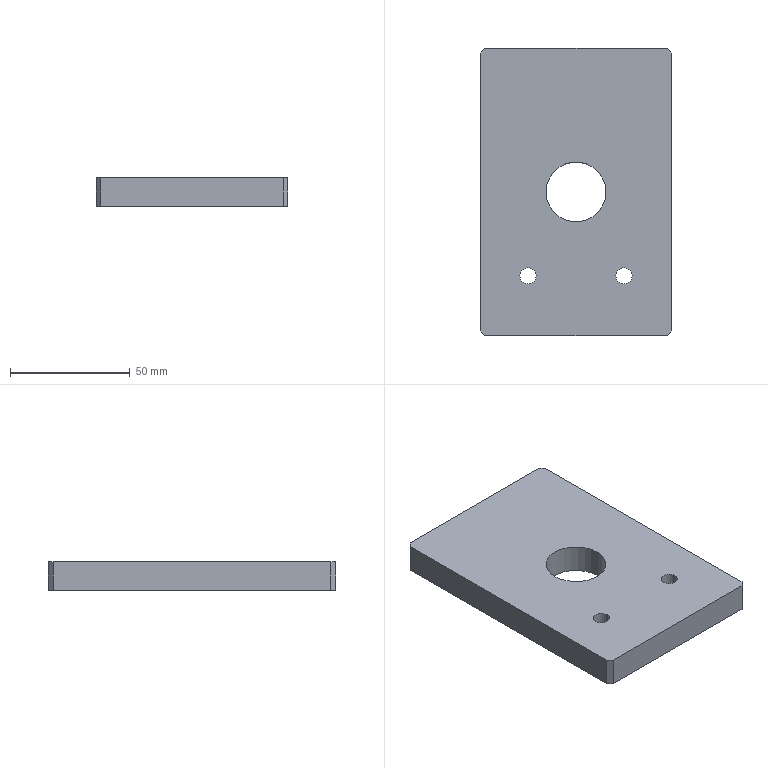Part | SolidWorks | features BaseBody 1 | 1 solid | 24 faces | box 80 x 120 x 12 mm | volume 106676 mm3 | cylinder 10 | plane 10 | cone 4 | commonest cylinder face diameters 6.8 x8 25 x2
STEP:
#1=CARTESIAN_POINT('',(12.5,0.,0.));
#2=VERTEX_POINT('',#1);
#3=CARTESIAN_POINT('',(-12.5,0.,0.));
#4=VERTEX_POINT('',#3);
#5=CARTESIAN_POINT('',(0.,0.,0.));
#6=DIRECTION('',(0.,0.,-1.));
#7=DIRECTION('',(1.,0.,0.));
#8=AXIS2_PLACEMENT_3D('',#5,#6,#7);
#9=CIRCLE('',#8,12.5);
#10=EDGE_CURVE('',#2,#4,#9,.T.);
#11=ORIENTED_EDGE('',*,*,#10,.T.);
#12=CARTESIAN_POINT('',(-12.5,0.,12.));
#13=VERTEX_POINT('',#12);
#14=CARTESIAN_POINT('',(-12.5,0.,0.));
#15=DIRECTION('',(0.,0.,1.));
#16=VECTOR('',#15,1000.);
#17=LINE('',#14,#16);
#18=EDGE_CURVE('',#4,#13,#17,.T.);
#19=ORIENTED_EDGE('',*,*,#18,.T.);
#20=CARTESIAN_POINT('',(12.5,0.,12.));
#21=VERTEX_POINT('',#20);
#22=CARTESIAN_POINT('',(0.,0.,12.));
#23=DIRECTION('',(0.,0.,-1.));
#24=DIRECTION('',(1.,0.,0.));
#25=AXIS2_PLACEMENT_3D('',#22,#23,#24);
#26=CIRCLE('',#25,12.5);
#27=EDGE_CURVE('',#21,#13,#26,.T.);
#28=ORIENTED_EDGE('',*,*,#27,.F.);
#29=CARTESIAN_POINT('',(12.5,0.,0.));
#30=DIRECTION('',(0.,0.,1.));
#31=VECTOR('',#30,1000.);
#32=LINE('',#29,#31);
#33=EDGE_CURVE('',#2,#21,#32,.T.);
#34=ORIENTED_EDGE('',*,*,#33,.F.);
#35=EDGE_LOOP('',(#11,#19,#28,#34));
#36=FACE_OUTER_BOUND('',#35,.T.);
#37=CARTESIAN_POINT('',(0.,0.,0.));
#38=DIRECTION('',(0.,0.,1.));
#39=DIRECTION('',(1.,0.,0.));
#40=AXIS2_PLACEMENT_3D('',#37,#38,#39);
#41=CYLINDRICAL_SURFACE('',#40,12.5);
#42=ADVANCED_FACE('',(#36),#41,.F.);
#43=CARTESIAN_POINT('',(-16.6,-35.,12.));
#44=VERTEX_POINT('',#43);
#45=CARTESIAN_POINT('',(-23.4,-35.,12.));
#46=VERTEX_POINT('',#45);
#47=CARTESIAN_POINT('',(-20.,-35.,12.));
#48=DIRECTION('',(0.,0.,-1.));
#49=DIRECTION('',(-1.,0.,0.));
#50=AXIS2_PLACEMENT_3D('',#47,#48,#49);
#51=CIRCLE('',#50,3.4);
#52=EDGE_CURVE('',#44,#46,#51,.T.);
#53=ORIENTED_EDGE('',*,*,#52,.F.);
#54=CARTESIAN_POINT('',(-16.6,-35.,0.));
#55=VERTEX_POINT('',#54);
#56=CARTESIAN_POINT('',(-16.6,-35.,0.));
#57=DIRECTION('',(0.,0.,-1.));
#58=VECTOR('',#57,1000.);
#59=LINE('',#56,#58);
#60=EDGE_CURVE('',#44,#55,#59,.T.);
#61=ORIENTED_EDGE('',*,*,#60,.T.);
#62=CARTESIAN_POINT('',(-23.4,-35.,0.));
#63=VERTEX_POINT('',#62);
#64=CARTESIAN_POINT('',(-20.,-35.,0.));
#65=DIRECTION('',(0.,0.,-1.));
#66=DIRECTION('',(-1.,0.,0.));
#67=AXIS2_PLACEMENT_3D('',#64,#65,#66);
#68=CIRCLE('',#67,3.4);
#69=EDGE_CURVE('',#55,#63,#68,.T.);
#70=ORIENTED_EDGE('',*,*,#69,.T.);
#71=CARTESIAN_POINT('',(-23.4,-35.,0.));
#72=DIRECTION('',(0.,0.,-1.));
#73=VECTOR('',#72,1000.);
#74=LINE('',#71,#73);
#75=EDGE_CURVE('',#46,#63,#74,.T.);
#76=ORIENTED_EDGE('',*,*,#75,.F.);
#77=EDGE_LOOP('',(#53,#61,#70,#76));
#78=FACE_OUTER_BOUND('',#77,.T.);
#79=CARTESIAN_POINT('',(-20.,-35.,0.));
#80=DIRECTION('',(0.,0.,-1.));
#81=DIRECTION('',(-1.,0.,0.));
#82=AXIS2_PLACEMENT_3D('',#79,#80,#81);
#83=CYLINDRICAL_SURFACE('',#82,3.4);
#84=ADVANCED_FACE('',(#78),#83,.F.);
#85=CARTESIAN_POINT('',(23.4,-35.,12.));
#86=VERTEX_POINT('',#85);
#87=CARTESIAN_POINT('',(16.6,-35.,12.));
#88=VERTEX_POINT('',#87);
#89=CARTESIAN_POINT('',(20.,-35.,12.));
#90=DIRECTION('',(0.,0.,-1.));
#91=DIRECTION('',(-1.,0.,0.));
#92=AXIS2_PLACEMENT_3D('',#89,#90,#91);
#93=CIRCLE('',#92,3.4);
#94=EDGE_CURVE('',#86,#88,#93,.T.);
#95=ORIENTED_EDGE('',*,*,#94,.F.);
#96=CARTESIAN_POINT('',(23.4,-35.,0.));
#97=VERTEX_POINT('',#96);
#98=CARTESIAN_POINT('',(23.4,-35.,0.));
#99=DIRECTION('',(0.,0.,-1.));
#100=VECTOR('',#99,1000.);
#101=LINE('',#98,#100);
#102=EDGE_CURVE('',#86,#97,#101,.T.);
#103=ORIENTED_EDGE('',*,*,#102,.T.);
#104=CARTESIAN_POINT('',(16.6,-35.,0.));
#105=VERTEX_POINT('',#104);
#106=CARTESIAN_POINT('',(20.,-35.,0.));
#107=DIRECTION('',(0.,0.,-1.));
#108=DIRECTION('',(-1.,0.,0.));
#109=AXIS2_PLACEMENT_3D('',#106,#107,#108);
#110=CIRCLE('',#109,3.4);
#111=EDGE_CURVE('',#97,#105,#110,.T.);
#112=ORIENTED_EDGE('',*,*,#111,.T.);
#113=CARTESIAN_POINT('',(16.6,-35.,0.));
#114=DIRECTION('',(0.,0.,-1.));
#115=VECTOR('',#114,1000.);
#116=LINE('',#113,#115);
#117=EDGE_CURVE('',#88,#105,#116,.T.);
#118=ORIENTED_EDGE('',*,*,#117,.F.);
#119=EDGE_LOOP('',(#95,#103,#112,#118));
#120=FACE_OUTER_BOUND('',#119,.T.);
#121=CARTESIAN_POINT('',(20.,-35.,0.));
#122=DIRECTION('',(0.,0.,-1.));
#123=DIRECTION('',(-1.,0.,0.));
#124=AXIS2_PLACEMENT_3D('',#121,#122,#123);
#125=CYLINDRICAL_SURFACE('',#124,3.4);
#126=ADVANCED_FACE('',(#120),#125,.F.);
#127=CARTESIAN_POINT('',(-20.,37.75,2.6));
#128=VERTEX_POINT('',#127);
#129=CARTESIAN_POINT('',(-20.,37.75,9.4));
#130=VERTEX_POINT('',#129);
#131=CARTESIAN_POINT('',(-20.,37.75,6.));
#132=DIRECTION('',(0.,1.,0.));
#133=DIRECTION('',(0.,0.,1.));
#134=AXIS2_PLACEMENT_3D('',#131,#132,#133);
#135=CIRCLE('',#134,3.4);
#136=EDGE_CURVE('',#128,#130,#135,.T.);
#137=ORIENTED_EDGE('',*,*,#136,.F.);
#138=CARTESIAN_POINT('',(-20.,60.,2.6));
#139=VERTEX_POINT('',#138);
#140=CARTESIAN_POINT('',(-20.,60.,2.6));
#141=DIRECTION('',(0.,1.,0.));
#142=VECTOR('',#141,1000.);
#143=LINE('',#140,#142);
#144=EDGE_CURVE('',#128,#139,#143,.T.);
#145=ORIENTED_EDGE('',*,*,#144,.T.);
#146=CARTESIAN_POINT('',(-20.,60.,9.4));
#147=VERTEX_POINT('',#146);
#148=CARTESIAN_POINT('',(-20.,60.,6.));
#149=DIRECTION('',(0.,1.,0.));
#150=DIRECTION('',(0.,0.,1.));
#151=AXIS2_PLACEMENT_3D('',#148,#149,#150);
#152=CIRCLE('',#151,3.4);
#153=EDGE_CURVE('',#139,#147,#152,.T.);
#154=ORIENTED_EDGE('',*,*,#153,.T.);
#155=CARTESIAN_POINT('',(-20.,60.,9.4));
#156=DIRECTION('',(0.,1.,0.));
#157=VECTOR('',#156,1000.);
#158=LINE('',#155,#157);
#159=EDGE_CURVE('',#130,#147,#158,.T.);
#160=ORIENTED_EDGE('',*,*,#159,.F.);
#161=EDGE_LOOP('',(#137,#145,#154,#160));
#162=FACE_OUTER_BOUND('',#161,.T.);
#163=CARTESIAN_POINT('',(-20.,60.,6.));
#164=DIRECTION('',(0.,1.,0.));
#165=DIRECTION('',(0.,0.,1.));
#166=AXIS2_PLACEMENT_3D('',#163,#164,#165);
#167=CYLINDRICAL_SURFACE('',#166,3.4);
#168=ADVANCED_FACE('',(#162),#167,.F.);
#169=CARTESIAN_POINT('',(20.,37.75,2.6));
#170=VERTEX_POINT('',#169);
#171=CARTESIAN_POINT('',(20.,37.75,9.4));
#172=VERTEX_POINT('',#171);
#173=CARTESIAN_POINT('',(20.,37.75,6.));
#174=DIRECTION('',(0.,1.,0.));
#175=DIRECTION('',(0.,0.,1.));
#176=AXIS2_PLACEMENT_3D('',#173,#174,#175);
#177=CIRCLE('',#176,3.4);
#178=EDGE_CURVE('',#170,#172,#177,.T.);
#179=ORIENTED_EDGE('',*,*,#178,.F.);
#180=CARTESIAN_POINT('',(20.,60.,2.6));
#181=VERTEX_POINT('',#180);
#182=CARTESIAN_POINT('',(20.,60.,2.6));
#183=DIRECTION('',(0.,1.,0.));
#184=VECTOR('',#183,1000.);
#185=LINE('',#182,#184);
#186=EDGE_CURVE('',#170,#181,#185,.T.);
#187=ORIENTED_EDGE('',*,*,#186,.T.);
#188=CARTESIAN_POINT('',(20.,60.,9.4));
#189=VERTEX_POINT('',#188);
#190=CARTESIAN_POINT('',(20.,60.,6.));
#191=DIRECTION('',(0.,1.,0.));
#192=DIRECTION('',(0.,0.,1.));
#193=AXIS2_PLACEMENT_3D('',#190,#191,#192);
#194=CIRCLE('',#193,3.4);
#195=EDGE_CURVE('',#181,#189,#194,.T.);
#196=ORIENTED_EDGE('',*,*,#195,.T.);
#197=CARTESIAN_POINT('',(20.,60.,9.4));
#198=DIRECTION('',(0.,1.,0.));
#199=VECTOR('',#198,1000.);
#200=LINE('',#197,#199);
#201=EDGE_CURVE('',#172,#189,#200,.T.);
#202=ORIENTED_EDGE('',*,*,#201,.F.);
#203=EDGE_LOOP('',(#179,#187,#196,#202));
#204=FACE_OUTER_BOUND('',#203,.T.);
#205=CARTESIAN_POINT('',(20.,60.,6.));
#206=DIRECTION('',(0.,1.,0.));
#207=DIRECTION('',(0.,0.,1.));
#208=AXIS2_PLACEMENT_3D('',#205,#206,#207);
#209=CYLINDRICAL_SURFACE('',#208,3.4);
#210=ADVANCED_FACE('',(#204),#209,.F.);
#211=CARTESIAN_POINT('',(-20.,35.707,6.));
#212=VERTEX_POINT('',#211);
#213=CARTESIAN_POINT('',(-20.,37.75,9.4));
#214=DIRECTION('',(0.,0.515,0.8572));
#215=VECTOR('',#214,1000.);
#216=LINE('',#213,#215);
#217=EDGE_CURVE('',#212,#130,#216,.T.);
#218=ORIENTED_EDGE('',*,*,#217,.F.);
#219=CARTESIAN_POINT('',(-20.,37.75,2.6));
#220=DIRECTION('',(0.,0.515,-0.8572));
#221=VECTOR('',#220,1000.);
#222=LINE('',#219,#221);
#223=EDGE_CURVE('',#212,#128,#222,.T.);
#224=ORIENTED_EDGE('',*,*,#223,.T.);
#225=ORIENTED_EDGE('',*,*,#136,.T.);
#226=EDGE_LOOP('',(#218,#224,#225));
#227=FACE_OUTER_BOUND('',#226,.T.);
#228=CARTESIAN_POINT('',(-20.,37.75,6.));
#229=DIRECTION('',(0.,1.,0.));
#230=DIRECTION('',(0.,0.,1.));
#231=AXIS2_PLACEMENT_3D('',#228,#229,#230);
#232=CONICAL_SURFACE('',#231,3.4,1.03);
#233=ADVANCED_FACE('',(#227),#232,.F.);
#234=CARTESIAN_POINT('',(20.,35.707,6.));
#235=VERTEX_POINT('',#234);
#236=CARTESIAN_POINT('',(20.,37.75,9.4));
#237=DIRECTION('',(0.,0.515,0.8572));
#238=VECTOR('',#237,1000.);
#239=LINE('',#236,#238);
#240=EDGE_CURVE('',#235,#172,#239,.T.);
#241=ORIENTED_EDGE('',*,*,#240,.F.);
#242=CARTESIAN_POINT('',(20.,37.75,2.6));
#243=DIRECTION('',(0.,0.515,-0.8572));
#244=VECTOR('',#243,1000.);
#245=LINE('',#242,#244);
#246=EDGE_CURVE('',#235,#170,#245,.T.);
#247=ORIENTED_EDGE('',*,*,#246,.T.);
#248=ORIENTED_EDGE('',*,*,#178,.T.);
#249=EDGE_LOOP('',(#241,#247,#248));
#250=FACE_OUTER_BOUND('',#249,.T.);
#251=CARTESIAN_POINT('',(20.,37.75,6.));
#252=DIRECTION('',(0.,1.,0.));
#253=DIRECTION('',(0.,0.,1.));
#254=AXIS2_PLACEMENT_3D('',#251,#252,#253);
#255=CONICAL_SURFACE('',#254,3.4,1.03);
#256=ADVANCED_FACE('',(#250),#255,.F.);
#257=CARTESIAN_POINT('',(-40.,-58.,0.));
#258=VERTEX_POINT('',#257);
#259=CARTESIAN_POINT('',(-38.,-60.,0.));
#260=VERTEX_POINT('',#259);
#261=CARTESIAN_POINT('',(-40.,-58.,0.));
#262=DIRECTION('',(0.7071,-0.7071,0.));
#263=VECTOR('',#262,1000.);
#264=LINE('',#261,#263);
#265=EDGE_CURVE('',#258,#260,#264,.T.);
#266=ORIENTED_EDGE('',*,*,#265,.F.);
#267=CARTESIAN_POINT('',(-40.,58.,0.));
#268=VERTEX_POINT('',#267);
#269=CARTESIAN_POINT('',(-40.,0.,0.));
#270=DIRECTION('',(0.,-1.,0.));
#271=VECTOR('',#270,1000.);
#272=LINE('',#269,#271);
#273=EDGE_CURVE('',#268,#258,#272,.T.);
#274=ORIENTED_EDGE('',*,*,#273,.F.);
#275=CARTESIAN_POINT('',(-38.,60.,0.));
#276=VERTEX_POINT('',#275);
#277=CARTESIAN_POINT('',(-38.,60.,0.));
#278=DIRECTION('',(-0.7071,-0.7071,0.));
#279=VECTOR('',#278,1000.);
#280=LINE('',#277,#279);
#281=EDGE_CURVE('',#276,#268,#280,.T.);
#282=ORIENTED_EDGE('',*,*,#281,.F.);
#283=CARTESIAN_POINT('',(38.,60.,0.));
#284=VERTEX_POINT('',#283);
#285=CARTESIAN_POINT('',(0.,60.,0.));
#286=DIRECTION('',(-1.,0.,0.));
#287=VECTOR('',#286,1000.);
#288=LINE('',#285,#287);
#289=EDGE_CURVE('',#284,#276,#288,.T.);
#290=ORIENTED_EDGE('',*,*,#289,.F.);
#291=CARTESIAN_POINT('',(40.,58.,0.));
#292=VERTEX_POINT('',#291);
#293=CARTESIAN_POINT('',(40.,58.,0.));
#294=DIRECTION('',(-0.7071,0.7071,0.));
#295=VECTOR('',#294,1000.);
#296=LINE('',#293,#295);
#297=EDGE_CURVE('',#292,#284,#296,.T.);
#298=ORIENTED_EDGE('',*,*,#297,.F.);
#299=CARTESIAN_POINT('',(40.,-58.,0.));
#300=VERTEX_POINT('',#299);
#301=CARTESIAN_POINT('',(40.,0.,0.));
#302=DIRECTION('',(0.,1.,0.));
#303=VECTOR('',#302,1000.);
#304=LINE('',#301,#303);
#305=EDGE_CURVE('',#300,#292,#304,.T.);
#306=ORIENTED_EDGE('',*,*,#305,.F.);
#307=CARTESIAN_POINT('',(38.,-60.,0.));
#308=VERTEX_POINT('',#307);
#309=CARTESIAN_POINT('',(38.,-60.,0.));
#310=DIRECTION('',(0.7071,0.7071,0.));
#311=VECTOR('',#310,1000.);
#312=LINE('',#309,#311);
#313=EDGE_CURVE('',#308,#300,#312,.T.);
#314=ORIENTED_EDGE('',*,*,#313,.F.);
#315=CARTESIAN_POINT('',(0.,-60.,0.));
#316=DIRECTION('',(1.,0.,0.));
#317=VECTOR('',#316,1000.);
#318=LINE('',#315,#317);
#319=EDGE_CURVE('',#260,#308,#318,.T.);
#320=ORIENTED_EDGE('',*,*,#319,.F.);
#321=EDGE_LOOP('',(#266,#274,#282,#290,#298,#306,#314,#320));
#322=FACE_OUTER_BOUND('',#321,.T.);
#323=ORIENTED_EDGE('',*,*,#10,.F.);
#324=CARTESIAN_POINT('',(0.,0.,0.));
#325=DIRECTION('',(0.,0.,-1.));
#326=DIRECTION('',(1.,0.,0.));
#327=AXIS2_PLACEMENT_3D('',#324,#325,#326);
#328=CIRCLE('',#327,12.5);
#329=EDGE_CURVE('',#4,#2,#328,.T.);
#330=ORIENTED_EDGE('',*,*,#329,.F.);
#331=EDGE_LOOP('',(#323,#330));
#332=FACE_BOUND('',#331,.T.);
#333=CARTESIAN_POINT('',(-20.,-35.,0.));
#334=DIRECTION('',(0.,0.,-1.));
#335=DIRECTION('',(-1.,0.,0.));
#336=AXIS2_PLACEMENT_3D('',#333,#334,#335);
#337=CIRCLE('',#336,3.4);
#338=EDGE_CURVE('',#63,#55,#337,.T.);
#339=ORIENTED_EDGE('',*,*,#338,.F.);
#340=ORIENTED_EDGE('',*,*,#69,.F.);
#341=EDGE_LOOP('',(#339,#340));
#342=FACE_BOUND('',#341,.T.);
#343=CARTESIAN_POINT('',(20.,-35.,0.));
#344=DIRECTION('',(0.,0.,-1.));
#345=DIRECTION('',(-1.,0.,0.));
#346=AXIS2_PLACEMENT_3D('',#343,#344,#345);
#347=CIRCLE('',#346,3.4);
#348=EDGE_CURVE('',#105,#97,#347,.T.);
#349=ORIENTED_EDGE('',*,*,#348,.F.);
#350=ORIENTED_EDGE('',*,*,#111,.F.);
#351=EDGE_LOOP('',(#349,#350));
#352=FACE_BOUND('',#351,.T.);
#353=CARTESIAN_POINT('',(0.,0.,0.));
#354=DIRECTION('',(0.,0.,1.));
#355=DIRECTION('',(1.,0.,0.));
#356=AXIS2_PLACEMENT_3D('',#353,#354,#355);
#357=PLANE('',#356);
#358=ADVANCED_FACE('',(#322,#332,#342,#352),#357,.F.);
#359=CARTESIAN_POINT('',(-38.,-60.,12.));
#360=VERTEX_POINT('',#359);
#361=CARTESIAN_POINT('',(-38.,-60.,12.));
#362=DIRECTION('',(0.,0.,1.));
#363=VECTOR('',#362,1000.);
#364=LINE('',#361,#363);
#365=EDGE_CURVE('',#260,#360,#364,.T.);
#366=ORIENTED_EDGE('',*,*,#365,.F.);
#367=ORIENTED_EDGE('',*,*,#319,.T.);
#368=CARTESIAN_POINT('',(38.,-60.,12.));
#369=VERTEX_POINT('',#368);
#370=CARTESIAN_POINT('',(38.,-60.,12.));
#371=DIRECTION('',(0.,0.,-1.));
#372=VECTOR('',#371,1000.);
#373=LINE('',#370,#372);
#374=EDGE_CURVE('',#369,#308,#373,.T.);
#375=ORIENTED_EDGE('',*,*,#374,.F.);
#376=CARTESIAN_POINT('',(-40.,-60.,12.));
#377=DIRECTION('',(1.,0.,0.));
#378=VECTOR('',#377,1000.);
#379=LINE('',#376,#378);
#380=EDGE_CURVE('',#360,#369,#379,.T.);
#381=ORIENTED_EDGE('',*,*,#380,.F.);
#382=EDGE_LOOP('',(#366,#367,#375,#381));
#383=FACE_OUTER_BOUND('',#382,.T.);
#384=CARTESIAN_POINT('',(-40.,-60.,12.));
#385=DIRECTION('',(0.,1.,0.));
#386=DIRECTION('',(0.,0.,1.));
#387=AXIS2_PLACEMENT_3D('',#384,#385,#386);
#388=PLANE('',#387);
#389=ADVANCED_FACE('',(#383),#388,.F.);
#390=CARTESIAN_POINT('',(-40.,-58.,12.));
#391=VERTEX_POINT('',#390);
#392=CARTESIAN_POINT('',(-40.,-58.,12.));
#393=DIRECTION('',(0.,0.,1.));
#394=VECTOR('',#393,1000.);
#395=LINE('',#392,#394);
#396=EDGE_CURVE('',#258,#391,#395,.T.);
#397=ORIENTED_EDGE('',*,*,#396,.F.);
#398=ORIENTED_EDGE('',*,*,#265,.T.);
#399=ORIENTED_EDGE('',*,*,#365,.T.);
#400=CARTESIAN_POINT('',(-38.,-60.,12.));
#401=DIRECTION('',(0.7071,-0.7071,0.));
#402=VECTOR('',#401,1000.);
#403=LINE('',#400,#402);
#404=EDGE_CURVE('',#391,#360,#403,.T.);
#405=ORIENTED_EDGE('',*,*,#404,.F.);
#406=EDGE_LOOP('',(#397,#398,#399,#405));
#407=FACE_OUTER_BOUND('',#406,.T.);
#408=CARTESIAN_POINT('',(-38.,-60.,12.));
#409=DIRECTION('',(0.7071,0.7071,0.));
#410=DIRECTION('',(-0.7071,0.7071,0.));
#411=AXIS2_PLACEMENT_3D('',#408,#409,#410);
#412=PLANE('',#411);
#413=ADVANCED_FACE('',(#407),#412,.F.);
#414=ORIENTED_EDGE('',*,*,#396,.T.);
#415=CARTESIAN_POINT('',(-40.,58.,12.));
#416=VERTEX_POINT('',#415);
#417=CARTESIAN_POINT('',(-40.,60.,12.));
#418=DIRECTION('',(0.,-1.,0.));
#419=VECTOR('',#418,1000.);
#420=LINE('',#417,#419);
#421=EDGE_CURVE('',#416,#391,#420,.T.);
#422=ORIENTED_EDGE('',*,*,#421,.F.);
#423=CARTESIAN_POINT('',(-40.,58.,12.));
#424=DIRECTION('',(0.,0.,1.));
#425=VECTOR('',#424,1000.);
#426=LINE('',#423,#425);
#427=EDGE_CURVE('',#268,#416,#426,.T.);
#428=ORIENTED_EDGE('',*,*,#427,.F.);
#429=ORIENTED_EDGE('',*,*,#273,.T.);
#430=EDGE_LOOP('',(#414,#422,#428,#429));
#431=FACE_OUTER_BOUND('',#430,.T.);
#432=CARTESIAN_POINT('',(-40.,60.,12.));
#433=DIRECTION('',(1.,0.,0.));
#434=DIRECTION('',(0.,1.,0.));
#435=AXIS2_PLACEMENT_3D('',#432,#433,#434);
#436=PLANE('',#435);
#437=ADVANCED_FACE('',(#431),#436,.F.);
#438=CARTESIAN_POINT('',(-38.,60.,12.));
#439=VERTEX_POINT('',#438);
#440=CARTESIAN_POINT('',(-38.,60.,12.));
#441=DIRECTION('',(0.,0.,1.));
#442=VECTOR('',#441,1000.);
#443=LINE('',#440,#442);
#444=EDGE_CURVE('',#276,#439,#443,.T.);
#445=ORIENTED_EDGE('',*,*,#444,.F.);
#446=ORIENTED_EDGE('',*,*,#281,.T.);
#447=ORIENTED_EDGE('',*,*,#427,.T.);
#448=CARTESIAN_POINT('',(-40.,58.,12.));
#449=DIRECTION('',(-0.7071,-0.7071,0.));
#450=VECTOR('',#449,1000.);
#451=LINE('',#448,#450);
#452=EDGE_CURVE('',#439,#416,#451,.T.);
#453=ORIENTED_EDGE('',*,*,#452,.F.);
#454=EDGE_LOOP('',(#445,#446,#447,#453));
#455=FACE_OUTER_BOUND('',#454,.T.);
#456=CARTESIAN_POINT('',(-40.,58.,12.));
#457=DIRECTION('',(0.7071,-0.7071,0.));
#458=DIRECTION('',(0.7071,0.7071,0.));
#459=AXIS2_PLACEMENT_3D('',#456,#457,#458);
#460=PLANE('',#459);
#461=ADVANCED_FACE('',(#455),#460,.F.);
#462=CARTESIAN_POINT('',(38.,60.,12.));
#463=VERTEX_POINT('',#462);
#464=CARTESIAN_POINT('',(38.,60.,12.));
#465=DIRECTION('',(0.,0.,1.));
#466=VECTOR('',#465,1000.);
#467=LINE('',#464,#466);
#468=EDGE_CURVE('',#284,#463,#467,.T.);
#469=ORIENTED_EDGE('',*,*,#468,.F.);
#470=ORIENTED_EDGE('',*,*,#289,.T.);
#471=ORIENTED_EDGE('',*,*,#444,.T.);
#472=CARTESIAN_POINT('',(-40.,60.,12.));
#473=DIRECTION('',(-1.,0.,0.));
#474=VECTOR('',#473,1000.);
#475=LINE('',#472,#474);
#476=EDGE_CURVE('',#463,#439,#475,.T.);
#477=ORIENTED_EDGE('',*,*,#476,.F.);
#478=EDGE_LOOP('',(#469,#470,#471,#477));
#479=FACE_OUTER_BOUND('',#478,.T.);
#480=CARTESIAN_POINT('',(-20.,60.,6.));
#481=DIRECTION('',(0.,1.,0.));
#482=DIRECTION('',(0.,0.,1.));
#483=AXIS2_PLACEMENT_3D('',#480,#481,#482);
#484=CIRCLE('',#483,3.4);
#485=EDGE_CURVE('',#147,#139,#484,.T.);
#486=ORIENTED_EDGE('',*,*,#485,.F.);
#487=ORIENTED_EDGE('',*,*,#153,.F.);
#488=EDGE_LOOP('',(#486,#487));
#489=FACE_BOUND('',#488,.T.);
#490=CARTESIAN_POINT('',(20.,60.,6.));
#491=DIRECTION('',(0.,1.,0.));
#492=DIRECTION('',(0.,0.,1.));
#493=AXIS2_PLACEMENT_3D('',#490,#491,#492);
#494=CIRCLE('',#493,3.4);
#495=EDGE_CURVE('',#189,#181,#494,.T.);
#496=ORIENTED_EDGE('',*,*,#495,.F.);
#497=ORIENTED_EDGE('',*,*,#195,.F.);
#498=EDGE_LOOP('',(#496,#497));
#499=FACE_BOUND('',#498,.T.);
#500=CARTESIAN_POINT('',(-40.,60.,12.));
#501=DIRECTION('',(0.,-1.,0.));
#502=DIRECTION('',(0.,0.,-1.));
#503=AXIS2_PLACEMENT_3D('',#500,#501,#502);
#504=PLANE('',#503);
#505=ADVANCED_FACE('',(#479,#489,#499),#504,.F.);
#506=CARTESIAN_POINT('',(40.,58.,12.));
#507=VERTEX_POINT('',#506);
#508=CARTESIAN_POINT('',(40.,58.,12.));
#509=DIRECTION('',(0.,0.,1.));
#510=VECTOR('',#509,1000.);
#511=LINE('',#508,#510);
#512=EDGE_CURVE('',#292,#507,#511,.T.);
#513=ORIENTED_EDGE('',*,*,#512,.F.);
#514=ORIENTED_EDGE('',*,*,#297,.T.);
#515=ORIENTED_EDGE('',*,*,#468,.T.);
#516=CARTESIAN_POINT('',(38.,60.,12.));
#517=DIRECTION('',(-0.7071,0.7071,0.));
#518=VECTOR('',#517,1000.);
#519=LINE('',#516,#518);
#520=EDGE_CURVE('',#507,#463,#519,.T.);
#521=ORIENTED_EDGE('',*,*,#520,.F.);
#522=EDGE_LOOP('',(#513,#514,#515,#521));
#523=FACE_OUTER_BOUND('',#522,.T.);
#524=CARTESIAN_POINT('',(38.,60.,12.));
#525=DIRECTION('',(-0.7071,-0.7071,0.));
#526=DIRECTION('',(0.7071,-0.7071,0.));
#527=AXIS2_PLACEMENT_3D('',#524,#525,#526);
#528=PLANE('',#527);
#529=ADVANCED_FACE('',(#523),#528,.F.);
#530=CARTESIAN_POINT('',(40.,-58.,12.));
#531=VERTEX_POINT('',#530);
#532=CARTESIAN_POINT('',(40.,-58.,12.));
#533=DIRECTION('',(0.,0.,1.));
#534=VECTOR('',#533,1000.);
#535=LINE('',#532,#534);
#536=EDGE_CURVE('',#300,#531,#535,.T.);
#537=ORIENTED_EDGE('',*,*,#536,.F.);
#538=ORIENTED_EDGE('',*,*,#305,.T.);
#539=ORIENTED_EDGE('',*,*,#512,.T.);
#540=CARTESIAN_POINT('',(40.,60.,12.));
#541=DIRECTION('',(0.,1.,0.));
#542=VECTOR('',#541,1000.);
#543=LINE('',#540,#542);
#544=EDGE_CURVE('',#531,#507,#543,.T.);
#545=ORIENTED_EDGE('',*,*,#544,.F.);
#546=EDGE_LOOP('',(#537,#538,#539,#545));
#547=FACE_OUTER_BOUND('',#546,.T.);
#548=CARTESIAN_POINT('',(40.,60.,12.));
#549=DIRECTION('',(-1.,0.,0.));
#550=DIRECTION('',(0.,-1.,0.));
#551=AXIS2_PLACEMENT_3D('',#548,#549,#550);
#552=PLANE('',#551);
#553=ADVANCED_FACE('',(#547),#552,.F.);
#554=ORIENTED_EDGE('',*,*,#374,.T.);
#555=ORIENTED_EDGE('',*,*,#313,.T.);
#556=ORIENTED_EDGE('',*,*,#536,.T.);
#557=CARTESIAN_POINT('',(40.,-58.,12.));
#558=DIRECTION('',(0.7071,0.7071,0.));
#559=VECTOR('',#558,1000.);
#560=LINE('',#557,#559);
#561=EDGE_CURVE('',#369,#531,#560,.T.);
#562=ORIENTED_EDGE('',*,*,#561,.F.);
#563=EDGE_LOOP('',(#554,#555,#556,#562));
#564=FACE_OUTER_BOUND('',#563,.T.);
#565=CARTESIAN_POINT('',(40.,-58.,12.));
#566=DIRECTION('',(-0.7071,0.7071,0.));
#567=DIRECTION('',(-0.7071,-0.7071,0.));
#568=AXIS2_PLACEMENT_3D('',#565,#566,#567);
#569=PLANE('',#568);
#570=ADVANCED_FACE('',(#564),#569,.F.);
#571=ORIENTED_EDGE('',*,*,#18,.F.);
#572=ORIENTED_EDGE('',*,*,#329,.T.);
#573=ORIENTED_EDGE('',*,*,#33,.T.);
#574=CARTESIAN_POINT('',(0.,0.,12.));
#575=DIRECTION('',(0.,0.,-1.));
#576=DIRECTION('',(1.,0.,0.));
#577=AXIS2_PLACEMENT_3D('',#574,#575,#576);
#578=CIRCLE('',#577,12.5);
#579=EDGE_CURVE('',#13,#21,#578,.T.);
#580=ORIENTED_EDGE('',*,*,#579,.F.);
#581=EDGE_LOOP('',(#571,#572,#573,#580));
#582=FACE_OUTER_BOUND('',#581,.T.);
#583=CARTESIAN_POINT('',(0.,0.,0.));
#584=DIRECTION('',(0.,0.,1.));
#585=DIRECTION('',(1.,0.,0.));
#586=AXIS2_PLACEMENT_3D('',#583,#584,#585);
#587=CYLINDRICAL_SURFACE('',#586,12.5);
#588=ADVANCED_FACE('',(#582),#587,.F.);
#589=ORIENTED_EDGE('',*,*,#60,.F.);
#590=CARTESIAN_POINT('',(-20.,-35.,12.));
#591=DIRECTION('',(0.,0.,-1.));
#592=DIRECTION('',(-1.,0.,0.));
#593=AXIS2_PLACEMENT_3D('',#590,#591,#592);
#594=CIRCLE('',#593,3.4);
#595=EDGE_CURVE('',#46,#44,#594,.T.);
#596=ORIENTED_EDGE('',*,*,#595,.F.);
#597=ORIENTED_EDGE('',*,*,#75,.T.);
#598=ORIENTED_EDGE('',*,*,#338,.T.);
#599=EDGE_LOOP('',(#589,#596,#597,#598));
#600=FACE_OUTER_BOUND('',#599,.T.);
#601=CARTESIAN_POINT('',(-20.,-35.,0.));
#602=DIRECTION('',(0.,0.,-1.));
#603=DIRECTION('',(-1.,0.,0.));
#604=AXIS2_PLACEMENT_3D('',#601,#602,#603);
#605=CYLINDRICAL_SURFACE('',#604,3.4);
#606=ADVANCED_FACE('',(#600),#605,.F.);
#607=ORIENTED_EDGE('',*,*,#102,.F.);
#608=CARTESIAN_POINT('',(20.,-35.,12.));
#609=DIRECTION('',(0.,0.,-1.));
#610=DIRECTION('',(-1.,0.,0.));
#611=AXIS2_PLACEMENT_3D('',#608,#609,#610);
#612=CIRCLE('',#611,3.4);
#613=EDGE_CURVE('',#88,#86,#612,.T.);
#614=ORIENTED_EDGE('',*,*,#613,.F.);
#615=ORIENTED_EDGE('',*,*,#117,.T.);
#616=ORIENTED_EDGE('',*,*,#348,.T.);
#617=EDGE_LOOP('',(#607,#614,#615,#616));
#618=FACE_OUTER_BOUND('',#617,.T.);
#619=CARTESIAN_POINT('',(20.,-35.,0.));
#620=DIRECTION('',(0.,0.,-1.));
#621=DIRECTION('',(-1.,0.,0.));
#622=AXIS2_PLACEMENT_3D('',#619,#620,#621);
#623=CYLINDRICAL_SURFACE('',#622,3.4);
#624=ADVANCED_FACE('',(#618),#623,.F.);
#625=ORIENTED_EDGE('',*,*,#476,.T.);
#626=ORIENTED_EDGE('',*,*,#452,.T.);
#627=ORIENTED_EDGE('',*,*,#421,.T.);
#628=ORIENTED_EDGE('',*,*,#404,.T.);
#629=ORIENTED_EDGE('',*,*,#380,.T.);
#630=ORIENTED_EDGE('',*,*,#561,.T.);
#631=ORIENTED_EDGE('',*,*,#544,.T.);
#632=ORIENTED_EDGE('',*,*,#520,.T.);
#633=EDGE_LOOP('',(#625,#626,#627,#628,#629,#630,#631,#632));
#634=FACE_OUTER_BOUND('',#633,.T.);
#635=ORIENTED_EDGE('',*,*,#27,.T.);
#636=ORIENTED_EDGE('',*,*,#579,.T.);
#637=EDGE_LOOP('',(#635,#636));
#638=FACE_BOUND('',#637,.T.);
#639=ORIENTED_EDGE('',*,*,#595,.T.);
#640=ORIENTED_EDGE('',*,*,#52,.T.);
#641=EDGE_LOOP('',(#639,#640));
#642=FACE_BOUND('',#641,.T.);
#643=ORIENTED_EDGE('',*,*,#613,.T.);
#644=ORIENTED_EDGE('',*,*,#94,.T.);
#645=EDGE_LOOP('',(#643,#644));
#646=FACE_BOUND('',#645,.T.);
#647=CARTESIAN_POINT('',(0.,0.,12.));
#648=DIRECTION('',(0.,0.,1.));
#649=DIRECTION('',(1.,0.,0.));
#650=AXIS2_PLACEMENT_3D('',#647,#648,#649);
#651=PLANE('',#650);
#652=ADVANCED_FACE('',(#634,#638,#642,#646),#651,.T.);
#653=ORIENTED_EDGE('',*,*,#144,.F.);
#654=CARTESIAN_POINT('',(-20.,37.75,6.));
#655=DIRECTION('',(0.,1.,0.));
#656=DIRECTION('',(0.,0.,1.));
#657=AXIS2_PLACEMENT_3D('',#654,#655,#656);
#658=CIRCLE('',#657,3.4);
#659=EDGE_CURVE('',#130,#128,#658,.T.);
#660=ORIENTED_EDGE('',*,*,#659,.F.);
#661=ORIENTED_EDGE('',*,*,#159,.T.);
#662=ORIENTED_EDGE('',*,*,#485,.T.);
#663=EDGE_LOOP('',(#653,#660,#661,#662));
#664=FACE_OUTER_BOUND('',#663,.T.);
#665=CARTESIAN_POINT('',(-20.,60.,6.));
#666=DIRECTION('',(0.,1.,0.));
#667=DIRECTION('',(0.,0.,1.));
#668=AXIS2_PLACEMENT_3D('',#665,#666,#667);
#669=CYLINDRICAL_SURFACE('',#668,3.4);
#670=ADVANCED_FACE('',(#664),#669,.F.);
#671=ORIENTED_EDGE('',*,*,#186,.F.);
#672=CARTESIAN_POINT('',(20.,37.75,6.));
#673=DIRECTION('',(0.,1.,0.));
#674=DIRECTION('',(0.,0.,1.));
#675=AXIS2_PLACEMENT_3D('',#672,#673,#674);
#676=CIRCLE('',#675,3.4);
#677=EDGE_CURVE('',#172,#170,#676,.T.);
#678=ORIENTED_EDGE('',*,*,#677,.F.);
#679=ORIENTED_EDGE('',*,*,#201,.T.);
#680=ORIENTED_EDGE('',*,*,#495,.T.);
#681=EDGE_LOOP('',(#671,#678,#679,#680));
#682=FACE_OUTER_BOUND('',#681,.T.);
#683=CARTESIAN_POINT('',(20.,60.,6.));
#684=DIRECTION('',(0.,1.,0.));
#685=DIRECTION('',(0.,0.,1.));
#686=AXIS2_PLACEMENT_3D('',#683,#684,#685);
#687=CYLINDRICAL_SURFACE('',#686,3.4);
#688=ADVANCED_FACE('',(#682),#687,.F.);
#689=ORIENTED_EDGE('',*,*,#223,.F.);
#690=ORIENTED_EDGE('',*,*,#217,.T.);
#691=ORIENTED_EDGE('',*,*,#659,.T.);
#692=EDGE_LOOP('',(#689,#690,#691));
#693=FACE_OUTER_BOUND('',#692,.T.);
#694=CARTESIAN_POINT('',(-20.,37.75,6.));
#695=DIRECTION('',(0.,1.,0.));
#696=DIRECTION('',(0.,0.,1.));
#697=AXIS2_PLACEMENT_3D('',#694,#695,#696);
#698=CONICAL_SURFACE('',#697,3.4,1.03);
#699=ADVANCED_FACE('',(#693),#698,.F.);
#700=ORIENTED_EDGE('',*,*,#246,.F.);
#701=ORIENTED_EDGE('',*,*,#240,.T.);
#702=ORIENTED_EDGE('',*,*,#677,.T.);
#703=EDGE_LOOP('',(#700,#701,#702));
#704=FACE_OUTER_BOUND('',#703,.T.);
#705=CARTESIAN_POINT('',(20.,37.75,6.));
#706=DIRECTION('',(0.,1.,0.));
#707=DIRECTION('',(0.,0.,1.));
#708=AXIS2_PLACEMENT_3D('',#705,#706,#707);
#709=CONICAL_SURFACE('',#708,3.4,1.03);
#710=ADVANCED_FACE('',(#704),#709,.F.);
#711=CLOSED_SHELL('',(#42,#84,#126,#168,#210,#233,#256,#358,#389,#413,#437,#461,#505,#529,#553,#570,#588,#606,#624,#652,#670,#688,#699,#710));
#712=MANIFOLD_SOLID_BREP('',#711);
#713=CARTESIAN_POINT('',(0.,0.,0.));
#714=DIRECTION('',(0.,0.,1.));
#715=DIRECTION('',(1.,0.,0.));
#716=AXIS2_PLACEMENT_3D('',#713,#714,#715);
#717=(LENGTH_UNIT()NAMED_UNIT(*)SI_UNIT(.MILLI.,.METRE.));
#718=UNCERTAINTY_MEASURE_WITH_UNIT(LENGTH_MEASURE(0.00001),#717,'','');
#719=(NAMED_UNIT(*)PLANE_ANGLE_UNIT()SI_UNIT($,.RADIAN.));
#720=(NAMED_UNIT(*)SI_UNIT($,.STERADIAN.)SOLID_ANGLE_UNIT());
#721=(GEOMETRIC_REPRESENTATION_CONTEXT(3)GLOBAL_UNCERTAINTY_ASSIGNED_CONTEXT((#718))GLOBAL_UNIT_ASSIGNED_CONTEXT((#717,#719,#720))REPRESENTATION_CONTEXT('',''));
#722=ADVANCED_BREP_SHAPE_REPRESENTATION('',(#712,#716),#721);